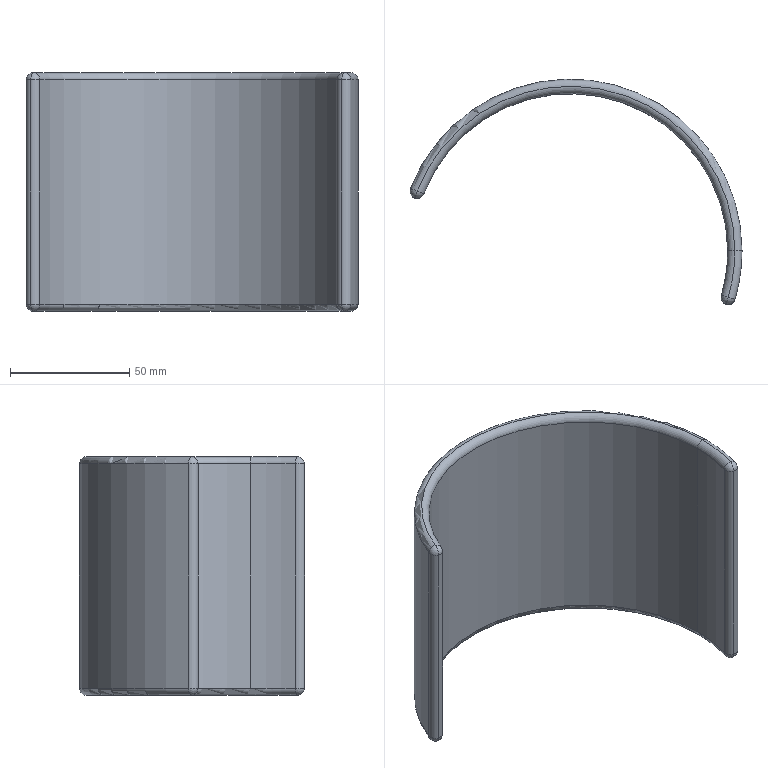Part | SolidWorks | features ICE 2, Extrusion 1, Fillet 1 | 1 solid | 22 faces | box 139.296 x 94.506 x 100 mm | volume 127694 mm3 | cylinder 8 | sphere 8 | torus 6 | commonest cylinder face diameters 6 x4 132 x2 144 x2
STEP:
#1=CARTESIAN_POINT('',(-159.216,103.149,39.5));
#2=VERTEX_POINT('',#1);
#3=CARTESIAN_POINT('',(-162.153,82.794,39.5));
#4=VERTEX_POINT('',#3);
#5=CARTESIAN_POINT('',(-231.216,103.149,39.5));
#6=DIRECTION('',(0.,0.,-1.));
#7=DIRECTION('',(1.,0.,0.));
#8=AXIS2_PLACEMENT_3D('',#5,#6,#7);
#9=CIRCLE('',#8,72.);
#10=EDGE_CURVE('',#2,#4,#9,.T.);
#11=ORIENTED_EDGE('',*,*,#10,.F.);
#12=CARTESIAN_POINT('',(-162.216,103.149,42.5));
#13=VERTEX_POINT('',#12);
#14=CARTESIAN_POINT('',(-162.216,103.149,39.5));
#15=DIRECTION('',(0.,-1.,0.));
#16=DIRECTION('',(0.,0.,-1.));
#17=AXIS2_PLACEMENT_3D('',#14,#15,#16);
#18=CIRCLE('',#17,3.);
#19=EDGE_CURVE('',#2,#13,#18,.T.);
#20=ORIENTED_EDGE('',*,*,#19,.T.);
#21=CARTESIAN_POINT('',(-165.031,83.643,42.5));
#22=VERTEX_POINT('',#21);
#23=CARTESIAN_POINT('',(-231.216,103.149,42.5));
#24=DIRECTION('',(0.,0.,-1.));
#25=DIRECTION('',(1.,0.,0.));
#26=AXIS2_PLACEMENT_3D('',#23,#24,#25);
#27=CIRCLE('',#26,69.);
#28=EDGE_CURVE('',#13,#22,#27,.T.);
#29=ORIENTED_EDGE('',*,*,#28,.T.);
#30=CARTESIAN_POINT('',(-165.031,83.643,39.5));
#31=DIRECTION('',(-0.2827,-0.9592,0.));
#32=DIRECTION('',(0.9592,-0.2827,0.));
#33=AXIS2_PLACEMENT_3D('',#30,#31,#32);
#34=CIRCLE('',#33,3.);
#35=EDGE_CURVE('',#4,#22,#34,.T.);
#36=ORIENTED_EDGE('',*,*,#35,.F.);
#37=EDGE_LOOP('',(#11,#20,#29,#36));
#38=FACE_OUTER_BOUND('',#37,.T.);
#39=CARTESIAN_POINT('',(-231.216,103.149,39.5));
#40=DIRECTION('',(0.,0.,1.));
#41=DIRECTION('',(1.,0.,0.));
#42=AXIS2_PLACEMENT_3D('',#39,#40,#41);
#43=TOROIDAL_SURFACE('',#42,69.,3.);
#44=ADVANCED_FACE('',(#38),#43,.T.);
#45=ORIENTED_EDGE('',*,*,#28,.F.);
#46=CARTESIAN_POINT('',(-165.216,103.149,39.5));
#47=VERTEX_POINT('',#46);
#48=CARTESIAN_POINT('',(-162.216,103.149,39.5));
#49=DIRECTION('',(0.,-1.,0.));
#50=DIRECTION('',(0.,0.,-1.));
#51=AXIS2_PLACEMENT_3D('',#48,#49,#50);
#52=CIRCLE('',#51,3.);
#53=EDGE_CURVE('',#13,#47,#52,.T.);
#54=ORIENTED_EDGE('',*,*,#53,.T.);
#55=CARTESIAN_POINT('',(-167.908,84.491,39.5));
#56=VERTEX_POINT('',#55);
#57=CARTESIAN_POINT('',(-231.216,103.149,39.5));
#58=DIRECTION('',(0.,0.,1.));
#59=DIRECTION('',(1.,0.,0.));
#60=AXIS2_PLACEMENT_3D('',#57,#58,#59);
#61=CIRCLE('',#60,66.);
#62=EDGE_CURVE('',#56,#47,#61,.T.);
#63=ORIENTED_EDGE('',*,*,#62,.F.);
#64=CARTESIAN_POINT('',(-165.031,83.643,39.5));
#65=DIRECTION('',(-0.2827,-0.9592,0.));
#66=DIRECTION('',(0.9592,-0.2827,0.));
#67=AXIS2_PLACEMENT_3D('',#64,#65,#66);
#68=CIRCLE('',#67,3.);
#69=EDGE_CURVE('',#22,#56,#68,.T.);
#70=ORIENTED_EDGE('',*,*,#69,.F.);
#71=EDGE_LOOP('',(#45,#54,#63,#70));
#72=FACE_OUTER_BOUND('',#71,.T.);
#73=CARTESIAN_POINT('',(-231.216,103.149,39.5));
#74=DIRECTION('',(0.,0.,1.));
#75=DIRECTION('',(1.,0.,0.));
#76=AXIS2_PLACEMENT_3D('',#73,#74,#75);
#77=TOROIDAL_SURFACE('',#76,69.,3.);
#78=ADVANCED_FACE('',(#72),#77,.T.);
#79=CARTESIAN_POINT('',(-162.153,82.794,-54.5));
#80=VERTEX_POINT('',#79);
#81=CARTESIAN_POINT('',(-159.216,103.149,-54.5));
#82=VERTEX_POINT('',#81);
#83=CARTESIAN_POINT('',(-231.216,103.149,-54.5));
#84=DIRECTION('',(0.,0.,1.));
#85=DIRECTION('',(-1.,0.,0.));
#86=AXIS2_PLACEMENT_3D('',#83,#84,#85);
#87=CIRCLE('',#86,72.);
#88=EDGE_CURVE('',#80,#82,#87,.T.);
#89=ORIENTED_EDGE('',*,*,#88,.T.);
#90=CARTESIAN_POINT('',(-159.216,103.149,-184.512));
#91=DIRECTION('',(0.,0.,1.));
#92=VECTOR('',#91,1000.);
#93=LINE('',#90,#92);
#94=EDGE_CURVE('',#82,#2,#93,.T.);
#95=ORIENTED_EDGE('',*,*,#94,.T.);
#96=ORIENTED_EDGE('',*,*,#10,.T.);
#97=CARTESIAN_POINT('',(-162.153,82.794,-184.512));
#98=DIRECTION('',(0.,0.,-1.));
#99=VECTOR('',#98,1000.);
#100=LINE('',#97,#99);
#101=EDGE_CURVE('',#4,#80,#100,.T.);
#102=ORIENTED_EDGE('',*,*,#101,.T.);
#103=EDGE_LOOP('',(#89,#95,#96,#102));
#104=FACE_OUTER_BOUND('',#103,.T.);
#105=CARTESIAN_POINT('',(-231.216,103.149,-184.512));
#106=DIRECTION('',(0.,0.,1.));
#107=DIRECTION('',(1.,0.,0.));
#108=AXIS2_PLACEMENT_3D('',#105,#106,#107);
#109=CYLINDRICAL_SURFACE('',#108,72.);
#110=ADVANCED_FACE('',(#104),#109,.T.);
#111=CARTESIAN_POINT('',(-292.717,127.1,-54.5));
#112=VERTEX_POINT('',#111);
#113=CARTESIAN_POINT('',(-165.216,103.149,-54.5));
#114=VERTEX_POINT('',#113);
#115=CARTESIAN_POINT('',(-231.216,103.149,-54.5));
#116=DIRECTION('',(0.,0.,-1.));
#117=DIRECTION('',(-1.,0.,0.));
#118=AXIS2_PLACEMENT_3D('',#115,#116,#117);
#119=CIRCLE('',#118,66.);
#120=EDGE_CURVE('',#112,#114,#119,.T.);
#121=ORIENTED_EDGE('',*,*,#120,.T.);
#122=CARTESIAN_POINT('',(-165.216,103.149,-184.512));
#123=DIRECTION('',(0.,0.,1.));
#124=VECTOR('',#123,1000.);
#125=LINE('',#122,#124);
#126=EDGE_CURVE('',#114,#47,#125,.T.);
#127=ORIENTED_EDGE('',*,*,#126,.T.);
#128=CARTESIAN_POINT('',(-292.717,127.1,39.5));
#129=VERTEX_POINT('',#128);
#130=CARTESIAN_POINT('',(-231.216,103.149,39.5));
#131=DIRECTION('',(0.,0.,1.));
#132=DIRECTION('',(1.,0.,0.));
#133=AXIS2_PLACEMENT_3D('',#130,#131,#132);
#134=CIRCLE('',#133,66.);
#135=EDGE_CURVE('',#47,#129,#134,.T.);
#136=ORIENTED_EDGE('',*,*,#135,.T.);
#137=CARTESIAN_POINT('',(-292.717,127.1,-184.512));
#138=DIRECTION('',(0.,0.,-1.));
#139=VECTOR('',#138,1000.);
#140=LINE('',#137,#139);
#141=EDGE_CURVE('',#129,#112,#140,.T.);
#142=ORIENTED_EDGE('',*,*,#141,.T.);
#143=EDGE_LOOP('',(#121,#127,#136,#142));
#144=FACE_OUTER_BOUND('',#143,.T.);
#145=CARTESIAN_POINT('',(-231.216,103.149,-184.512));
#146=DIRECTION('',(0.,0.,1.));
#147=DIRECTION('',(1.,0.,0.));
#148=AXIS2_PLACEMENT_3D('',#145,#146,#147);
#149=CYLINDRICAL_SURFACE('',#148,66.);
#150=ADVANCED_FACE('',(#144),#149,.F.);
#151=ORIENTED_EDGE('',*,*,#126,.F.);
#152=CARTESIAN_POINT('',(-167.908,84.491,-54.5));
#153=VERTEX_POINT('',#152);
#154=CARTESIAN_POINT('',(-231.216,103.149,-54.5));
#155=DIRECTION('',(0.,0.,-1.));
#156=DIRECTION('',(-1.,0.,0.));
#157=AXIS2_PLACEMENT_3D('',#154,#155,#156);
#158=CIRCLE('',#157,66.);
#159=EDGE_CURVE('',#114,#153,#158,.T.);
#160=ORIENTED_EDGE('',*,*,#159,.T.);
#161=CARTESIAN_POINT('',(-167.908,84.491,-184.512));
#162=DIRECTION('',(0.,0.,1.));
#163=VECTOR('',#162,1000.);
#164=LINE('',#161,#163);
#165=EDGE_CURVE('',#153,#56,#164,.T.);
#166=ORIENTED_EDGE('',*,*,#165,.T.);
#167=ORIENTED_EDGE('',*,*,#62,.T.);
#168=EDGE_LOOP('',(#151,#160,#166,#167));
#169=FACE_OUTER_BOUND('',#168,.T.);
#170=CARTESIAN_POINT('',(-231.216,103.149,-184.512));
#171=DIRECTION('',(0.,0.,1.));
#172=DIRECTION('',(1.,0.,0.));
#173=AXIS2_PLACEMENT_3D('',#170,#171,#172);
#174=CYLINDRICAL_SURFACE('',#173,66.);
#175=ADVANCED_FACE('',(#169),#174,.F.);
#176=ORIENTED_EDGE('',*,*,#94,.F.);
#177=CARTESIAN_POINT('',(-298.308,129.277,-54.5));
#178=VERTEX_POINT('',#177);
#179=CARTESIAN_POINT('',(-231.216,103.149,-54.5));
#180=DIRECTION('',(0.,0.,1.));
#181=DIRECTION('',(-1.,0.,0.));
#182=AXIS2_PLACEMENT_3D('',#179,#180,#181);
#183=CIRCLE('',#182,72.);
#184=EDGE_CURVE('',#82,#178,#183,.T.);
#185=ORIENTED_EDGE('',*,*,#184,.T.);
#186=CARTESIAN_POINT('',(-298.308,129.277,39.5));
#187=VERTEX_POINT('',#186);
#188=CARTESIAN_POINT('',(-298.308,129.277,-184.512));
#189=DIRECTION('',(0.,0.,1.));
#190=VECTOR('',#189,1000.);
#191=LINE('',#188,#190);
#192=EDGE_CURVE('',#178,#187,#191,.T.);
#193=ORIENTED_EDGE('',*,*,#192,.T.);
#194=CARTESIAN_POINT('',(-231.216,103.149,39.5));
#195=DIRECTION('',(0.,0.,-1.));
#196=DIRECTION('',(1.,0.,0.));
#197=AXIS2_PLACEMENT_3D('',#194,#195,#196);
#198=CIRCLE('',#197,72.);
#199=EDGE_CURVE('',#187,#2,#198,.T.);
#200=ORIENTED_EDGE('',*,*,#199,.T.);
#201=EDGE_LOOP('',(#176,#185,#193,#200));
#202=FACE_OUTER_BOUND('',#201,.T.);
#203=CARTESIAN_POINT('',(-231.216,103.149,-184.512));
#204=DIRECTION('',(0.,0.,1.));
#205=DIRECTION('',(1.,0.,0.));
#206=AXIS2_PLACEMENT_3D('',#203,#204,#205);
#207=CYLINDRICAL_SURFACE('',#206,72.);
#208=ADVANCED_FACE('',(#202),#207,.T.);
#209=ORIENTED_EDGE('',*,*,#53,.F.);
#210=CARTESIAN_POINT('',(-295.513,128.188,42.5));
#211=VERTEX_POINT('',#210);
#212=CARTESIAN_POINT('',(-231.216,103.149,42.5));
#213=DIRECTION('',(0.,0.,-1.));
#214=DIRECTION('',(1.,0.,0.));
#215=AXIS2_PLACEMENT_3D('',#212,#213,#214);
#216=CIRCLE('',#215,69.);
#217=EDGE_CURVE('',#211,#13,#216,.T.);
#218=ORIENTED_EDGE('',*,*,#217,.F.);
#219=CARTESIAN_POINT('',(-295.513,128.188,39.5));
#220=DIRECTION('',(-0.3629,-0.9318,0.));
#221=DIRECTION('',(0.9318,-0.3629,0.));
#222=AXIS2_PLACEMENT_3D('',#219,#220,#221);
#223=CIRCLE('',#222,3.);
#224=EDGE_CURVE('',#129,#211,#223,.T.);
#225=ORIENTED_EDGE('',*,*,#224,.F.);
#226=ORIENTED_EDGE('',*,*,#135,.F.);
#227=EDGE_LOOP('',(#209,#218,#225,#226));
#228=FACE_OUTER_BOUND('',#227,.T.);
#229=CARTESIAN_POINT('',(-231.216,103.149,39.5));
#230=DIRECTION('',(0.,0.,1.));
#231=DIRECTION('',(1.,0.,0.));
#232=AXIS2_PLACEMENT_3D('',#229,#230,#231);
#233=TOROIDAL_SURFACE('',#232,69.,3.);
#234=ADVANCED_FACE('',(#228),#233,.T.);
#235=ORIENTED_EDGE('',*,*,#224,.T.);
#236=CARTESIAN_POINT('',(-296.482,125.349,39.5));
#237=VERTEX_POINT('',#236);
#238=CARTESIAN_POINT('',(-295.513,128.188,39.5));
#239=DIRECTION('',(-0.9464,0.3231,0.));
#240=DIRECTION('',(-0.3231,-0.9464,0.));
#241=AXIS2_PLACEMENT_3D('',#238,#239,#240);
#242=CIRCLE('',#241,3.);
#243=EDGE_CURVE('',#237,#211,#242,.T.);
#244=ORIENTED_EDGE('',*,*,#243,.F.);
#245=CARTESIAN_POINT('',(-295.513,128.188,39.5));
#246=DIRECTION('',(0.,0.,-1.));
#247=DIRECTION('',(1.,0.,0.));
#248=AXIS2_PLACEMENT_3D('',#245,#246,#247);
#249=CIRCLE('',#248,3.);
#250=EDGE_CURVE('',#129,#237,#249,.T.);
#251=ORIENTED_EDGE('',*,*,#250,.F.);
#252=EDGE_LOOP('',(#235,#244,#251));
#253=FACE_OUTER_BOUND('',#252,.T.);
#254=CARTESIAN_POINT('',(-295.513,128.188,39.5));
#255=DIRECTION('',(0.,1.,0.));
#256=DIRECTION('',(1.,0.,0.));
#257=AXIS2_PLACEMENT_3D('',#254,#255,#256);
#258=SPHERICAL_SURFACE('',#257,3.);
#259=ADVANCED_FACE('',(#253),#258,.T.);
#260=CARTESIAN_POINT('',(-166.,80.803,39.5));
#261=VERTEX_POINT('',#260);
#262=CARTESIAN_POINT('',(-165.031,83.643,39.5));
#263=DIRECTION('',(0.9464,-0.3231,0.));
#264=DIRECTION('',(-0.3231,-0.9464,0.));
#265=AXIS2_PLACEMENT_3D('',#262,#263,#264);
#266=CIRCLE('',#265,3.);
#267=EDGE_CURVE('',#22,#261,#266,.T.);
#268=ORIENTED_EDGE('',*,*,#267,.F.);
#269=ORIENTED_EDGE('',*,*,#69,.T.);
#270=CARTESIAN_POINT('',(-165.031,83.643,39.5));
#271=DIRECTION('',(0.,0.,-1.));
#272=DIRECTION('',(0.,-1.,0.));
#273=AXIS2_PLACEMENT_3D('',#270,#271,#272);
#274=CIRCLE('',#273,3.);
#275=EDGE_CURVE('',#261,#56,#274,.T.);
#276=ORIENTED_EDGE('',*,*,#275,.F.);
#277=EDGE_LOOP('',(#268,#269,#276));
#278=FACE_OUTER_BOUND('',#277,.T.);
#279=CARTESIAN_POINT('',(-165.031,83.643,39.5));
#280=DIRECTION('',(0.,1.,0.));
#281=DIRECTION('',(1.,0.,0.));
#282=AXIS2_PLACEMENT_3D('',#279,#280,#281);
#283=SPHERICAL_SURFACE('',#282,3.);
#284=ADVANCED_FACE('',(#278),#283,.T.);
#285=ORIENTED_EDGE('',*,*,#19,.F.);
#286=ORIENTED_EDGE('',*,*,#199,.F.);
#287=CARTESIAN_POINT('',(-295.513,128.188,39.5));
#288=DIRECTION('',(-0.3629,-0.9318,0.));
#289=DIRECTION('',(0.9318,-0.3629,0.));
#290=AXIS2_PLACEMENT_3D('',#287,#288,#289);
#291=CIRCLE('',#290,3.);
#292=EDGE_CURVE('',#211,#187,#291,.T.);
#293=ORIENTED_EDGE('',*,*,#292,.F.);
#294=ORIENTED_EDGE('',*,*,#217,.T.);
#295=EDGE_LOOP('',(#285,#286,#293,#294));
#296=FACE_OUTER_BOUND('',#295,.T.);
#297=CARTESIAN_POINT('',(-231.216,103.149,39.5));
#298=DIRECTION('',(0.,0.,1.));
#299=DIRECTION('',(1.,0.,0.));
#300=AXIS2_PLACEMENT_3D('',#297,#298,#299);
#301=TOROIDAL_SURFACE('',#300,69.,3.);
#302=ADVANCED_FACE('',(#296),#301,.T.);
#303=ORIENTED_EDGE('',*,*,#243,.T.);
#304=ORIENTED_EDGE('',*,*,#292,.T.);
#305=CARTESIAN_POINT('',(-295.513,128.188,39.5));
#306=DIRECTION('',(0.,0.,-1.));
#307=DIRECTION('',(0.,-1.,0.));
#308=AXIS2_PLACEMENT_3D('',#305,#306,#307);
#309=CIRCLE('',#308,3.);
#310=EDGE_CURVE('',#237,#187,#309,.T.);
#311=ORIENTED_EDGE('',*,*,#310,.F.);
#312=EDGE_LOOP('',(#303,#304,#311));
#313=FACE_OUTER_BOUND('',#312,.T.);
#314=CARTESIAN_POINT('',(-295.513,128.188,39.5));
#315=DIRECTION('',(0.,1.,0.));
#316=DIRECTION('',(1.,0.,0.));
#317=AXIS2_PLACEMENT_3D('',#314,#315,#316);
#318=SPHERICAL_SURFACE('',#317,3.);
#319=ADVANCED_FACE('',(#313),#318,.T.);
#320=ORIENTED_EDGE('',*,*,#141,.F.);
#321=ORIENTED_EDGE('',*,*,#250,.T.);
#322=CARTESIAN_POINT('',(-296.482,125.349,-54.5));
#323=VERTEX_POINT('',#322);
#324=CARTESIAN_POINT('',(-296.482,125.349,-184.512));
#325=DIRECTION('',(0.,0.,1.));
#326=VECTOR('',#325,1000.);
#327=LINE('',#324,#326);
#328=EDGE_CURVE('',#323,#237,#327,.T.);
#329=ORIENTED_EDGE('',*,*,#328,.F.);
#330=CARTESIAN_POINT('',(-295.513,128.188,-54.5));
#331=DIRECTION('',(0.,0.,-1.));
#332=DIRECTION('',(0.,1.,0.));
#333=AXIS2_PLACEMENT_3D('',#330,#331,#332);
#334=CIRCLE('',#333,3.);
#335=EDGE_CURVE('',#112,#323,#334,.T.);
#336=ORIENTED_EDGE('',*,*,#335,.F.);
#337=EDGE_LOOP('',(#320,#321,#329,#336));
#338=FACE_OUTER_BOUND('',#337,.T.);
#339=CARTESIAN_POINT('',(-295.513,128.188,-184.512));
#340=DIRECTION('',(0.,0.,1.));
#341=DIRECTION('',(1.,0.,0.));
#342=AXIS2_PLACEMENT_3D('',#339,#340,#341);
#343=CYLINDRICAL_SURFACE('',#342,3.);
#344=ADVANCED_FACE('',(#338),#343,.T.);
#345=ORIENTED_EDGE('',*,*,#275,.T.);
#346=ORIENTED_EDGE('',*,*,#165,.F.);
#347=CARTESIAN_POINT('',(-166.,80.803,-54.5));
#348=VERTEX_POINT('',#347);
#349=CARTESIAN_POINT('',(-165.031,83.643,-54.5));
#350=DIRECTION('',(0.,0.,-1.));
#351=DIRECTION('',(-1.,0.,0.));
#352=AXIS2_PLACEMENT_3D('',#349,#350,#351);
#353=CIRCLE('',#352,3.);
#354=EDGE_CURVE('',#348,#153,#353,.T.);
#355=ORIENTED_EDGE('',*,*,#354,.F.);
#356=CARTESIAN_POINT('',(-166.,80.803,-184.512));
#357=DIRECTION('',(0.,0.,-1.));
#358=VECTOR('',#357,1000.);
#359=LINE('',#356,#358);
#360=EDGE_CURVE('',#261,#348,#359,.T.);
#361=ORIENTED_EDGE('',*,*,#360,.F.);
#362=EDGE_LOOP('',(#345,#346,#355,#361));
#363=FACE_OUTER_BOUND('',#362,.T.);
#364=CARTESIAN_POINT('',(-165.031,83.643,-184.512));
#365=DIRECTION('',(0.,0.,1.));
#366=DIRECTION('',(1.,0.,0.));
#367=AXIS2_PLACEMENT_3D('',#364,#365,#366);
#368=CYLINDRICAL_SURFACE('',#367,3.);
#369=ADVANCED_FACE('',(#363),#368,.T.);
#370=ORIENTED_EDGE('',*,*,#35,.T.);
#371=ORIENTED_EDGE('',*,*,#267,.T.);
#372=CARTESIAN_POINT('',(-165.031,83.643,39.5));
#373=DIRECTION('',(0.,0.,-1.));
#374=DIRECTION('',(1.,0.,0.));
#375=AXIS2_PLACEMENT_3D('',#372,#373,#374);
#376=CIRCLE('',#375,3.);
#377=EDGE_CURVE('',#4,#261,#376,.T.);
#378=ORIENTED_EDGE('',*,*,#377,.F.);
#379=EDGE_LOOP('',(#370,#371,#378));
#380=FACE_OUTER_BOUND('',#379,.T.);
#381=CARTESIAN_POINT('',(-165.031,83.643,39.5));
#382=DIRECTION('',(0.,1.,0.));
#383=DIRECTION('',(1.,0.,0.));
#384=AXIS2_PLACEMENT_3D('',#381,#382,#383);
#385=SPHERICAL_SURFACE('',#384,3.);
#386=ADVANCED_FACE('',(#380),#385,.T.);
#387=CARTESIAN_POINT('',(-295.513,128.188,-54.5));
#388=DIRECTION('',(0.,0.,-1.));
#389=DIRECTION('',(-1.,0.,0.));
#390=AXIS2_PLACEMENT_3D('',#387,#388,#389);
#391=CIRCLE('',#390,3.);
#392=EDGE_CURVE('',#323,#178,#391,.T.);
#393=ORIENTED_EDGE('',*,*,#392,.F.);
#394=ORIENTED_EDGE('',*,*,#328,.T.);
#395=ORIENTED_EDGE('',*,*,#310,.T.);
#396=ORIENTED_EDGE('',*,*,#192,.F.);
#397=EDGE_LOOP('',(#393,#394,#395,#396));
#398=FACE_OUTER_BOUND('',#397,.T.);
#399=CARTESIAN_POINT('',(-295.513,128.188,-184.512));
#400=DIRECTION('',(0.,0.,1.));
#401=DIRECTION('',(1.,0.,0.));
#402=AXIS2_PLACEMENT_3D('',#399,#400,#401);
#403=CYLINDRICAL_SURFACE('',#402,3.);
#404=ADVANCED_FACE('',(#398),#403,.T.);
#405=ORIENTED_EDGE('',*,*,#335,.T.);
#406=CARTESIAN_POINT('',(-295.513,128.188,-57.5));
#407=VERTEX_POINT('',#406);
#408=CARTESIAN_POINT('',(-295.513,128.188,-54.5));
#409=DIRECTION('',(-0.9464,0.3231,0.));
#410=DIRECTION('',(-0.3231,-0.9464,0.));
#411=AXIS2_PLACEMENT_3D('',#408,#409,#410);
#412=CIRCLE('',#411,3.);
#413=EDGE_CURVE('',#407,#323,#412,.T.);
#414=ORIENTED_EDGE('',*,*,#413,.F.);
#415=CARTESIAN_POINT('',(-295.513,128.188,-54.5));
#416=DIRECTION('',(0.3629,0.9318,0.));
#417=DIRECTION('',(0.9318,-0.3629,0.));
#418=AXIS2_PLACEMENT_3D('',#415,#416,#417);
#419=CIRCLE('',#418,3.);
#420=EDGE_CURVE('',#112,#407,#419,.T.);
#421=ORIENTED_EDGE('',*,*,#420,.F.);
#422=EDGE_LOOP('',(#405,#414,#421));
#423=FACE_OUTER_BOUND('',#422,.T.);
#424=CARTESIAN_POINT('',(-295.513,128.188,-54.5));
#425=DIRECTION('',(0.,1.,0.));
#426=DIRECTION('',(1.,0.,0.));
#427=AXIS2_PLACEMENT_3D('',#424,#425,#426);
#428=SPHERICAL_SURFACE('',#427,3.);
#429=ADVANCED_FACE('',(#423),#428,.T.);
#430=CARTESIAN_POINT('',(-165.031,83.643,-57.5));
#431=VERTEX_POINT('',#430);
#432=CARTESIAN_POINT('',(-165.031,83.643,-54.5));
#433=DIRECTION('',(0.9464,-0.3231,0.));
#434=DIRECTION('',(-0.3231,-0.9464,0.));
#435=AXIS2_PLACEMENT_3D('',#432,#433,#434);
#436=CIRCLE('',#435,3.);
#437=EDGE_CURVE('',#348,#431,#436,.T.);
#438=ORIENTED_EDGE('',*,*,#437,.F.);
#439=ORIENTED_EDGE('',*,*,#354,.T.);
#440=CARTESIAN_POINT('',(-165.031,83.643,-54.5));
#441=DIRECTION('',(0.2827,0.9592,0.));
#442=DIRECTION('',(0.9592,-0.2827,0.));
#443=AXIS2_PLACEMENT_3D('',#440,#441,#442);
#444=CIRCLE('',#443,3.);
#445=EDGE_CURVE('',#431,#153,#444,.T.);
#446=ORIENTED_EDGE('',*,*,#445,.F.);
#447=EDGE_LOOP('',(#438,#439,#446));
#448=FACE_OUTER_BOUND('',#447,.T.);
#449=CARTESIAN_POINT('',(-165.031,83.643,-54.5));
#450=DIRECTION('',(0.,1.,0.));
#451=DIRECTION('',(1.,0.,0.));
#452=AXIS2_PLACEMENT_3D('',#449,#450,#451);
#453=SPHERICAL_SURFACE('',#452,3.);
#454=ADVANCED_FACE('',(#448),#453,.T.);
#455=ORIENTED_EDGE('',*,*,#377,.T.);
#456=ORIENTED_EDGE('',*,*,#360,.T.);
#457=CARTESIAN_POINT('',(-165.031,83.643,-54.5));
#458=DIRECTION('',(0.,0.,-1.));
#459=DIRECTION('',(0.,1.,0.));
#460=AXIS2_PLACEMENT_3D('',#457,#458,#459);
#461=CIRCLE('',#460,3.);
#462=EDGE_CURVE('',#80,#348,#461,.T.);
#463=ORIENTED_EDGE('',*,*,#462,.F.);
#464=ORIENTED_EDGE('',*,*,#101,.F.);
#465=EDGE_LOOP('',(#455,#456,#463,#464));
#466=FACE_OUTER_BOUND('',#465,.T.);
#467=CARTESIAN_POINT('',(-165.031,83.643,-184.512));
#468=DIRECTION('',(0.,0.,1.));
#469=DIRECTION('',(1.,0.,0.));
#470=AXIS2_PLACEMENT_3D('',#467,#468,#469);
#471=CYLINDRICAL_SURFACE('',#470,3.);
#472=ADVANCED_FACE('',(#466),#471,.T.);
#473=ORIENTED_EDGE('',*,*,#413,.T.);
#474=ORIENTED_EDGE('',*,*,#392,.T.);
#475=CARTESIAN_POINT('',(-295.513,128.188,-54.5));
#476=DIRECTION('',(0.3629,0.9318,0.));
#477=DIRECTION('',(0.9318,-0.3629,0.));
#478=AXIS2_PLACEMENT_3D('',#475,#476,#477);
#479=CIRCLE('',#478,3.);
#480=EDGE_CURVE('',#407,#178,#479,.T.);
#481=ORIENTED_EDGE('',*,*,#480,.F.);
#482=EDGE_LOOP('',(#473,#474,#481));
#483=FACE_OUTER_BOUND('',#482,.T.);
#484=CARTESIAN_POINT('',(-295.513,128.188,-54.5));
#485=DIRECTION('',(0.,1.,0.));
#486=DIRECTION('',(1.,0.,0.));
#487=AXIS2_PLACEMENT_3D('',#484,#485,#486);
#488=SPHERICAL_SURFACE('',#487,3.);
#489=ADVANCED_FACE('',(#483),#488,.T.);
#490=ORIENTED_EDGE('',*,*,#120,.F.);
#491=ORIENTED_EDGE('',*,*,#420,.T.);
#492=CARTESIAN_POINT('',(-231.216,103.149,-57.5));
#493=DIRECTION('',(0.,0.,1.));
#494=DIRECTION('',(-1.,0.,0.));
#495=AXIS2_PLACEMENT_3D('',#492,#493,#494);
#496=CIRCLE('',#495,69.);
#497=EDGE_CURVE('',#431,#407,#496,.T.);
#498=ORIENTED_EDGE('',*,*,#497,.F.);
#499=ORIENTED_EDGE('',*,*,#445,.T.);
#500=ORIENTED_EDGE('',*,*,#159,.F.);
#501=EDGE_LOOP('',(#490,#491,#498,#499,#500));
#502=FACE_OUTER_BOUND('',#501,.T.);
#503=CARTESIAN_POINT('',(-231.216,103.149,-54.5));
#504=DIRECTION('',(0.,0.,-1.));
#505=DIRECTION('',(-1.,0.,0.));
#506=AXIS2_PLACEMENT_3D('',#503,#504,#505);
#507=TOROIDAL_SURFACE('',#506,69.,3.);
#508=ADVANCED_FACE('',(#502),#507,.T.);
#509=ORIENTED_EDGE('',*,*,#462,.T.);
#510=ORIENTED_EDGE('',*,*,#437,.T.);
#511=CARTESIAN_POINT('',(-165.031,83.643,-54.5));
#512=DIRECTION('',(0.2827,0.9592,0.));
#513=DIRECTION('',(0.9592,-0.2827,0.));
#514=AXIS2_PLACEMENT_3D('',#511,#512,#513);
#515=CIRCLE('',#514,3.);
#516=EDGE_CURVE('',#80,#431,#515,.T.);
#517=ORIENTED_EDGE('',*,*,#516,.F.);
#518=EDGE_LOOP('',(#509,#510,#517));
#519=FACE_OUTER_BOUND('',#518,.T.);
#520=CARTESIAN_POINT('',(-165.031,83.643,-54.5));
#521=DIRECTION('',(0.,1.,0.));
#522=DIRECTION('',(1.,0.,0.));
#523=AXIS2_PLACEMENT_3D('',#520,#521,#522);
#524=SPHERICAL_SURFACE('',#523,3.);
#525=ADVANCED_FACE('',(#519),#524,.T.);
#526=ORIENTED_EDGE('',*,*,#480,.T.);
#527=ORIENTED_EDGE('',*,*,#184,.F.);
#528=ORIENTED_EDGE('',*,*,#88,.F.);
#529=ORIENTED_EDGE('',*,*,#516,.T.);
#530=ORIENTED_EDGE('',*,*,#497,.T.);
#531=EDGE_LOOP('',(#526,#527,#528,#529,#530));
#532=FACE_OUTER_BOUND('',#531,.T.);
#533=CARTESIAN_POINT('',(-231.216,103.149,-54.5));
#534=DIRECTION('',(0.,0.,-1.));
#535=DIRECTION('',(-1.,0.,0.));
#536=AXIS2_PLACEMENT_3D('',#533,#534,#535);
#537=TOROIDAL_SURFACE('',#536,69.,3.);
#538=ADVANCED_FACE('',(#532),#537,.T.);
#539=CLOSED_SHELL('',(#44,#78,#110,#150,#175,#208,#234,#259,#284,#302,#319,#344,#369,#386,#404,#429,#454,#472,#489,#508,#525,#538));
#540=MANIFOLD_SOLID_BREP('',#539);
#541=CARTESIAN_POINT('',(0.,0.,0.));
#542=DIRECTION('',(0.,0.,1.));
#543=DIRECTION('',(1.,0.,0.));
#544=AXIS2_PLACEMENT_3D('',#541,#542,#543);
#545=(LENGTH_UNIT()NAMED_UNIT(*)SI_UNIT(.MILLI.,.METRE.));
#546=UNCERTAINTY_MEASURE_WITH_UNIT(LENGTH_MEASURE(0.00001),#545,'','');
#547=(NAMED_UNIT(*)PLANE_ANGLE_UNIT()SI_UNIT($,.RADIAN.));
#548=(NAMED_UNIT(*)SI_UNIT($,.STERADIAN.)SOLID_ANGLE_UNIT());
#549=(GEOMETRIC_REPRESENTATION_CONTEXT(3)GLOBAL_UNCERTAINTY_ASSIGNED_CONTEXT((#546))GLOBAL_UNIT_ASSIGNED_CONTEXT((#545,#547,#548))REPRESENTATION_CONTEXT('',''));
#550=ADVANCED_BREP_SHAPE_REPRESENTATION('',(#540,#544),#549);